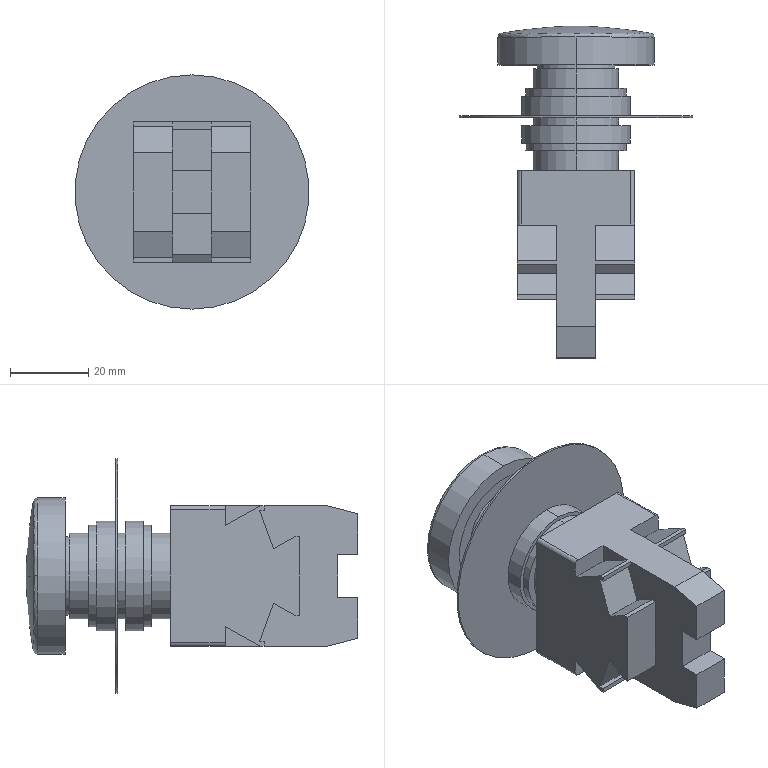Part | STEP file | Guide wheel mechanism revised.sldasm-Part-335 | 1 solid | 1404 faces | box 60 x 85 x 60 mm | volume 60625 mm3 | plane 1374 | cylinder 26 | spline 4 | commonest cylinder face diameters 22 x6 2 x4 26 x4 28 x4 20 x2 32 x2